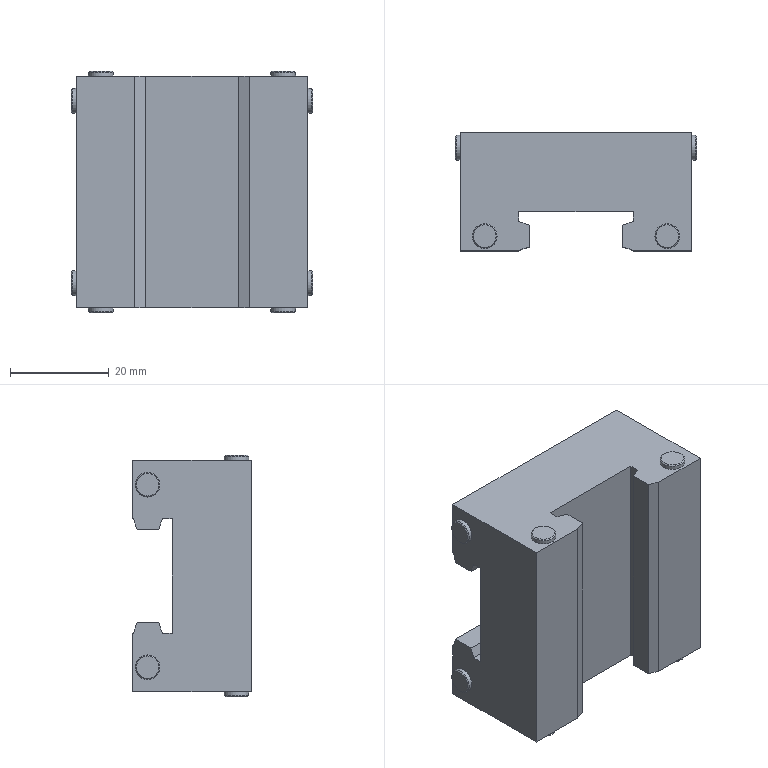Part | STEP file | 1 solid | 54 faces | box 49 x 24 x 49 mm | volume 37752 mm3 | plane 38 | cylinder 8 | cone 8 | commonest cylinder face diameters 5 x8